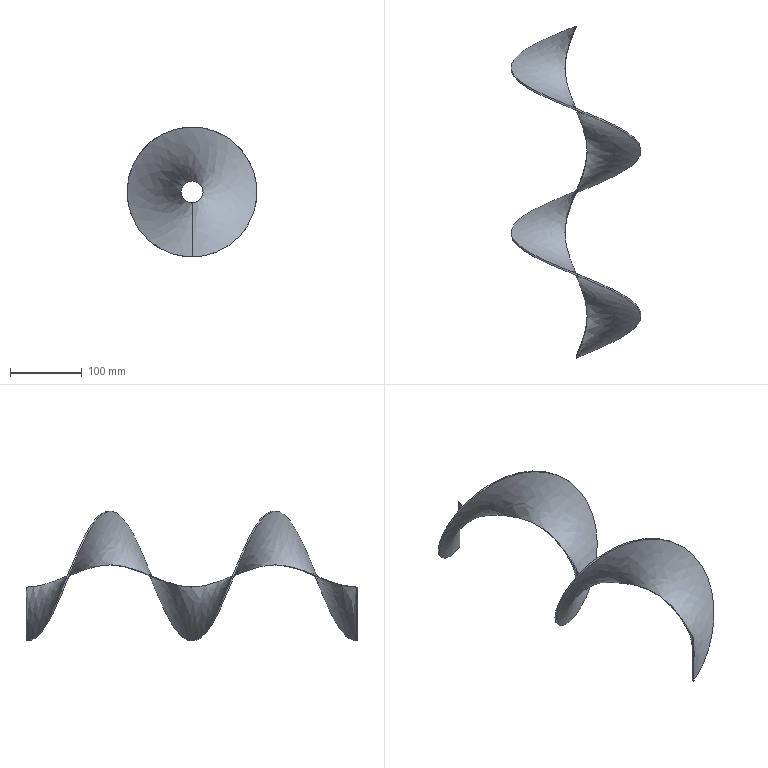Part | SolidWorks | features Helix 1, Sweep 1 | 1 solid | 6 faces | box 181 x 462.5 x 181 mm | volume 124893 mm3 | spline 4 | plane 2